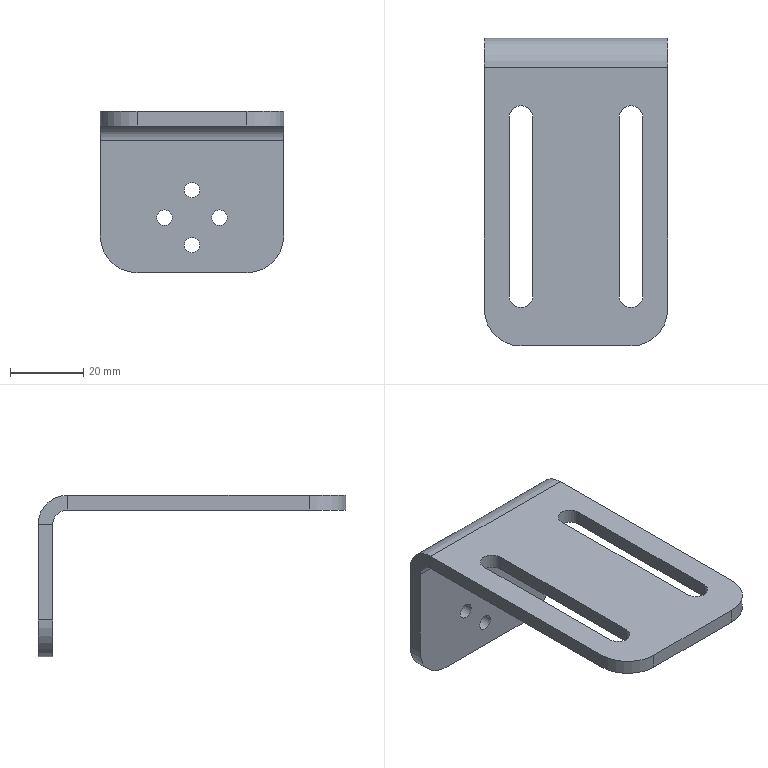Part | STEP file | JBJ-P-1010-04 | 1 solid | 30 faces | box 50 x 84 x 44 mm | volume 20932 mm3 | plane 16 | cylinder 14 | commonest cylinder face diameters 4.2 x4 6.5 x4 20 x4 8 x1 16 x1
STEP:
#1=CARTESIAN_POINT('',(50.,-4.,40.));
#2=VERTEX_POINT('',#1);
#3=CARTESIAN_POINT('',(50.,-4.,44.));
#4=VERTEX_POINT('',#3);
#5=CARTESIAN_POINT('',(50.,-4.,40.));
#6=DIRECTION('',(0.,0.,1.));
#7=VECTOR('',#6,1000.);
#8=LINE('',#5,#7);
#9=EDGE_CURVE('',#2,#4,#8,.T.);
#10=ORIENTED_EDGE('',*,*,#9,.F.);
#11=CARTESIAN_POINT('',(50.,0.,36.));
#12=VERTEX_POINT('',#11);
#13=CARTESIAN_POINT('',(50.,-4.,36.));
#14=DIRECTION('',(1.,0.,0.));
#15=DIRECTION('',(0.,0.,1.));
#16=AXIS2_PLACEMENT_3D('',#13,#14,#15);
#17=CIRCLE('',#16,4.);
#18=EDGE_CURVE('',#12,#2,#17,.T.);
#19=ORIENTED_EDGE('',*,*,#18,.F.);
#20=CARTESIAN_POINT('',(50.,4.,36.));
#21=VERTEX_POINT('',#20);
#22=CARTESIAN_POINT('',(50.,4.,36.));
#23=DIRECTION('',(0.,-1.,0.));
#24=VECTOR('',#23,1000.);
#25=LINE('',#22,#24);
#26=EDGE_CURVE('',#21,#12,#25,.T.);
#27=ORIENTED_EDGE('',*,*,#26,.F.);
#28=CARTESIAN_POINT('',(50.,-4.,36.));
#29=DIRECTION('',(1.,0.,0.));
#30=DIRECTION('',(0.,0.,-1.));
#31=AXIS2_PLACEMENT_3D('',#28,#29,#30);
#32=CIRCLE('',#31,8.);
#33=EDGE_CURVE('',#21,#4,#32,.T.);
#34=ORIENTED_EDGE('',*,*,#33,.T.);
#35=EDGE_LOOP('',(#10,#19,#27,#34));
#36=FACE_OUTER_BOUND('',#35,.T.);
#37=CARTESIAN_POINT('',(50.,-4.,40.));
#38=DIRECTION('',(1.,0.,0.));
#39=DIRECTION('',(0.,0.,-1.));
#40=AXIS2_PLACEMENT_3D('',#37,#38,#39);
#41=PLANE('',#40);
#42=ADVANCED_FACE('',(#36),#41,.T.);
#43=CARTESIAN_POINT('',(50.,-70.,44.));
#44=VERTEX_POINT('',#43);
#45=CARTESIAN_POINT('',(50.,0.,44.));
#46=DIRECTION('',(0.,-1.,0.));
#47=VECTOR('',#46,1000.);
#48=LINE('',#45,#47);
#49=EDGE_CURVE('',#4,#44,#48,.T.);
#50=ORIENTED_EDGE('',*,*,#49,.T.);
#51=CARTESIAN_POINT('',(50.,-70.,40.));
#52=VERTEX_POINT('',#51);
#53=CARTESIAN_POINT('',(50.,-70.,36.));
#54=DIRECTION('',(0.,0.,-1.));
#55=VECTOR('',#54,1000.);
#56=LINE('',#53,#55);
#57=EDGE_CURVE('',#44,#52,#56,.T.);
#58=ORIENTED_EDGE('',*,*,#57,.T.);
#59=CARTESIAN_POINT('',(50.,0.,40.));
#60=DIRECTION('',(0.,-1.,0.));
#61=VECTOR('',#60,1000.);
#62=LINE('',#59,#61);
#63=EDGE_CURVE('',#2,#52,#62,.T.);
#64=ORIENTED_EDGE('',*,*,#63,.F.);
#65=ORIENTED_EDGE('',*,*,#9,.T.);
#66=EDGE_LOOP('',(#50,#58,#64,#65));
#67=FACE_OUTER_BOUND('',#66,.T.);
#68=CARTESIAN_POINT('',(50.,4.,36.));
#69=DIRECTION('',(1.,0.,0.));
#70=DIRECTION('',(0.,0.,-1.));
#71=AXIS2_PLACEMENT_3D('',#68,#69,#70);
#72=PLANE('',#71);
#73=ADVANCED_FACE('',(#67),#72,.T.);
#74=CARTESIAN_POINT('',(0.,0.,36.));
#75=VERTEX_POINT('',#74);
#76=CARTESIAN_POINT('',(0.,4.,36.));
#77=VERTEX_POINT('',#76);
#78=CARTESIAN_POINT('',(0.,0.,36.));
#79=DIRECTION('',(0.,1.,0.));
#80=VECTOR('',#79,1000.);
#81=LINE('',#78,#80);
#82=EDGE_CURVE('',#75,#77,#81,.T.);
#83=ORIENTED_EDGE('',*,*,#82,.F.);
#84=CARTESIAN_POINT('',(0.,-4.,40.));
#85=VERTEX_POINT('',#84);
#86=CARTESIAN_POINT('',(0.,-4.,36.));
#87=DIRECTION('',(1.,0.,0.));
#88=DIRECTION('',(0.,0.,1.));
#89=AXIS2_PLACEMENT_3D('',#86,#87,#88);
#90=CIRCLE('',#89,4.);
#91=EDGE_CURVE('',#75,#85,#90,.T.);
#92=ORIENTED_EDGE('',*,*,#91,.T.);
#93=CARTESIAN_POINT('',(0.,-4.,44.));
#94=VERTEX_POINT('',#93);
#95=CARTESIAN_POINT('',(0.,-4.,44.));
#96=DIRECTION('',(0.,0.,-1.));
#97=VECTOR('',#96,1000.);
#98=LINE('',#95,#97);
#99=EDGE_CURVE('',#94,#85,#98,.T.);
#100=ORIENTED_EDGE('',*,*,#99,.F.);
#101=CARTESIAN_POINT('',(0.,-4.,36.));
#102=DIRECTION('',(1.,0.,0.));
#103=DIRECTION('',(0.,0.,-1.));
#104=AXIS2_PLACEMENT_3D('',#101,#102,#103);
#105=CIRCLE('',#104,8.);
#106=EDGE_CURVE('',#77,#94,#105,.T.);
#107=ORIENTED_EDGE('',*,*,#106,.F.);
#108=EDGE_LOOP('',(#83,#92,#100,#107));
#109=FACE_OUTER_BOUND('',#108,.T.);
#110=CARTESIAN_POINT('',(0.,0.,36.));
#111=DIRECTION('',(-1.,0.,0.));
#112=DIRECTION('',(0.,0.,1.));
#113=AXIS2_PLACEMENT_3D('',#110,#111,#112);
#114=PLANE('',#113);
#115=ADVANCED_FACE('',(#109),#114,.T.);
#116=CARTESIAN_POINT('',(0.,4.,10.));
#117=VERTEX_POINT('',#116);
#118=CARTESIAN_POINT('',(0.,4.,0.));
#119=DIRECTION('',(0.,0.,1.));
#120=VECTOR('',#119,1000.);
#121=LINE('',#118,#120);
#122=EDGE_CURVE('',#117,#77,#121,.T.);
#123=ORIENTED_EDGE('',*,*,#122,.F.);
#124=CARTESIAN_POINT('',(0.,0.,10.));
#125=VERTEX_POINT('',#124);
#126=CARTESIAN_POINT('',(0.,-4.,10.));
#127=DIRECTION('',(0.,-1.,0.));
#128=VECTOR('',#127,1000.);
#129=LINE('',#126,#128);
#130=EDGE_CURVE('',#117,#125,#129,.T.);
#131=ORIENTED_EDGE('',*,*,#130,.T.);
#132=CARTESIAN_POINT('',(0.,0.,0.));
#133=DIRECTION('',(0.,0.,1.));
#134=VECTOR('',#133,1000.);
#135=LINE('',#132,#134);
#136=EDGE_CURVE('',#125,#75,#135,.T.);
#137=ORIENTED_EDGE('',*,*,#136,.T.);
#138=ORIENTED_EDGE('',*,*,#82,.T.);
#139=EDGE_LOOP('',(#123,#131,#137,#138));
#140=FACE_OUTER_BOUND('',#139,.T.);
#141=CARTESIAN_POINT('',(0.,-4.,44.));
#142=DIRECTION('',(-1.,0.,0.));
#143=DIRECTION('',(0.,0.,1.));
#144=AXIS2_PLACEMENT_3D('',#141,#142,#143);
#145=PLANE('',#144);
#146=ADVANCED_FACE('',(#140),#145,.T.);
#147=CARTESIAN_POINT('',(36.75,-17.75,44.));
#148=VERTEX_POINT('',#147);
#149=CARTESIAN_POINT('',(43.25,-17.75,44.));
#150=VERTEX_POINT('',#149);
#151=CARTESIAN_POINT('',(40.,-17.75,44.));
#152=DIRECTION('',(0.,0.,-1.));
#153=DIRECTION('',(0.,1.,0.));
#154=AXIS2_PLACEMENT_3D('',#151,#152,#153);
#155=CIRCLE('',#154,3.25);
#156=EDGE_CURVE('',#148,#150,#155,.T.);
#157=ORIENTED_EDGE('',*,*,#156,.T.);
#158=CARTESIAN_POINT('',(43.25,-66.25,44.));
#159=VERTEX_POINT('',#158);
#160=CARTESIAN_POINT('',(43.25,-17.75,44.));
#161=DIRECTION('',(0.,-1.,0.));
#162=VECTOR('',#161,1000.);
#163=LINE('',#160,#162);
#164=EDGE_CURVE('',#150,#159,#163,.T.);
#165=ORIENTED_EDGE('',*,*,#164,.T.);
#166=CARTESIAN_POINT('',(36.75,-66.25,44.));
#167=VERTEX_POINT('',#166);
#168=CARTESIAN_POINT('',(40.,-66.25,44.));
#169=DIRECTION('',(0.,0.,-1.));
#170=DIRECTION('',(0.,1.,0.));
#171=AXIS2_PLACEMENT_3D('',#168,#169,#170);
#172=CIRCLE('',#171,3.25);
#173=EDGE_CURVE('',#159,#167,#172,.T.);
#174=ORIENTED_EDGE('',*,*,#173,.T.);
#175=CARTESIAN_POINT('',(36.75,-17.75,44.));
#176=DIRECTION('',(0.,-1.,0.));
#177=VECTOR('',#176,1000.);
#178=LINE('',#175,#177);
#179=EDGE_CURVE('',#148,#167,#178,.T.);
#180=ORIENTED_EDGE('',*,*,#179,.F.);
#181=EDGE_LOOP('',(#157,#165,#174,#180));
#182=FACE_BOUND('',#181,.T.);
#183=CARTESIAN_POINT('',(6.75,-17.75,44.));
#184=VERTEX_POINT('',#183);
#185=CARTESIAN_POINT('',(6.75,-66.25,44.));
#186=VERTEX_POINT('',#185);
#187=CARTESIAN_POINT('',(6.75,-17.75,44.));
#188=DIRECTION('',(0.,-1.,0.));
#189=VECTOR('',#188,1000.);
#190=LINE('',#187,#189);
#191=EDGE_CURVE('',#184,#186,#190,.T.);
#192=ORIENTED_EDGE('',*,*,#191,.F.);
#193=CARTESIAN_POINT('',(13.25,-17.75,44.));
#194=VERTEX_POINT('',#193);
#195=CARTESIAN_POINT('',(10.,-17.75,44.));
#196=DIRECTION('',(0.,0.,-1.));
#197=DIRECTION('',(0.,1.,0.));
#198=AXIS2_PLACEMENT_3D('',#195,#196,#197);
#199=CIRCLE('',#198,3.25);
#200=EDGE_CURVE('',#184,#194,#199,.T.);
#201=ORIENTED_EDGE('',*,*,#200,.T.);
#202=CARTESIAN_POINT('',(13.25,-66.25,44.));
#203=VERTEX_POINT('',#202);
#204=CARTESIAN_POINT('',(13.25,-17.75,44.));
#205=DIRECTION('',(0.,-1.,0.));
#206=VECTOR('',#205,1000.);
#207=LINE('',#204,#206);
#208=EDGE_CURVE('',#194,#203,#207,.T.);
#209=ORIENTED_EDGE('',*,*,#208,.T.);
#210=CARTESIAN_POINT('',(10.,-66.25,44.));
#211=DIRECTION('',(0.,0.,-1.));
#212=DIRECTION('',(0.,1.,0.));
#213=AXIS2_PLACEMENT_3D('',#210,#211,#212);
#214=CIRCLE('',#213,3.25);
#215=EDGE_CURVE('',#203,#186,#214,.T.);
#216=ORIENTED_EDGE('',*,*,#215,.T.);
#217=EDGE_LOOP('',(#192,#201,#209,#216));
#218=FACE_BOUND('',#217,.T.);
#219=CARTESIAN_POINT('',(40.,-80.,44.));
#220=VERTEX_POINT('',#219);
#221=CARTESIAN_POINT('',(10.,-80.,44.));
#222=VERTEX_POINT('',#221);
#223=CARTESIAN_POINT('',(50.,-80.,44.));
#224=DIRECTION('',(-1.,0.,0.));
#225=VECTOR('',#224,1000.);
#226=LINE('',#223,#225);
#227=EDGE_CURVE('',#220,#222,#226,.T.);
#228=ORIENTED_EDGE('',*,*,#227,.F.);
#229=CARTESIAN_POINT('',(40.,-70.,44.));
#230=DIRECTION('',(0.,0.,1.));
#231=DIRECTION('',(0.,1.,0.));
#232=AXIS2_PLACEMENT_3D('',#229,#230,#231);
#233=CIRCLE('',#232,10.);
#234=EDGE_CURVE('',#220,#44,#233,.T.);
#235=ORIENTED_EDGE('',*,*,#234,.T.);
#236=ORIENTED_EDGE('',*,*,#49,.F.);
#237=CARTESIAN_POINT('',(50.,-4.,44.));
#238=DIRECTION('',(-1.,0.,0.));
#239=VECTOR('',#238,1000.);
#240=LINE('',#237,#239);
#241=EDGE_CURVE('',#4,#94,#240,.T.);
#242=ORIENTED_EDGE('',*,*,#241,.T.);
#243=CARTESIAN_POINT('',(0.,-70.,44.));
#244=VERTEX_POINT('',#243);
#245=CARTESIAN_POINT('',(0.,0.,44.));
#246=DIRECTION('',(0.,-1.,0.));
#247=VECTOR('',#246,1000.);
#248=LINE('',#245,#247);
#249=EDGE_CURVE('',#94,#244,#248,.T.);
#250=ORIENTED_EDGE('',*,*,#249,.T.);
#251=CARTESIAN_POINT('',(10.,-70.,44.));
#252=DIRECTION('',(0.,0.,1.));
#253=DIRECTION('',(0.,1.,0.));
#254=AXIS2_PLACEMENT_3D('',#251,#252,#253);
#255=CIRCLE('',#254,10.);
#256=EDGE_CURVE('',#244,#222,#255,.T.);
#257=ORIENTED_EDGE('',*,*,#256,.T.);
#258=EDGE_LOOP('',(#228,#235,#236,#242,#250,#257));
#259=FACE_OUTER_BOUND('',#258,.T.);
#260=CARTESIAN_POINT('',(50.,0.,44.));
#261=DIRECTION('',(0.,0.,-1.));
#262=DIRECTION('',(0.,1.,0.));
#263=AXIS2_PLACEMENT_3D('',#260,#261,#262);
#264=PLANE('',#263);
#265=ADVANCED_FACE('',(#182,#218,#259),#264,.F.);
#266=CARTESIAN_POINT('',(40.,-80.,40.));
#267=VERTEX_POINT('',#266);
#268=CARTESIAN_POINT('',(10.,-80.,40.));
#269=VERTEX_POINT('',#268);
#270=CARTESIAN_POINT('',(50.,-80.,40.));
#271=DIRECTION('',(-1.,0.,0.));
#272=VECTOR('',#271,1000.);
#273=LINE('',#270,#272);
#274=EDGE_CURVE('',#267,#269,#273,.T.);
#275=ORIENTED_EDGE('',*,*,#274,.F.);
#276=CARTESIAN_POINT('',(40.,-80.,40.));
#277=DIRECTION('',(0.,0.,1.));
#278=VECTOR('',#277,1000.);
#279=LINE('',#276,#278);
#280=EDGE_CURVE('',#267,#220,#279,.T.);
#281=ORIENTED_EDGE('',*,*,#280,.T.);
#282=ORIENTED_EDGE('',*,*,#227,.T.);
#283=CARTESIAN_POINT('',(10.,-80.,40.));
#284=DIRECTION('',(0.,0.,-1.));
#285=VECTOR('',#284,1000.);
#286=LINE('',#283,#285);
#287=EDGE_CURVE('',#222,#269,#286,.T.);
#288=ORIENTED_EDGE('',*,*,#287,.T.);
#289=EDGE_LOOP('',(#275,#281,#282,#288));
#290=FACE_OUTER_BOUND('',#289,.T.);
#291=CARTESIAN_POINT('',(50.,-80.,40.));
#292=DIRECTION('',(0.,-1.,0.));
#293=DIRECTION('',(0.,0.,-1.));
#294=AXIS2_PLACEMENT_3D('',#291,#292,#293);
#295=PLANE('',#294);
#296=ADVANCED_FACE('',(#290),#295,.T.);
#297=CARTESIAN_POINT('',(36.75,-17.75,40.));
#298=VERTEX_POINT('',#297);
#299=CARTESIAN_POINT('',(36.75,-66.25,40.));
#300=VERTEX_POINT('',#299);
#301=CARTESIAN_POINT('',(36.75,-17.75,40.));
#302=DIRECTION('',(0.,-1.,0.));
#303=VECTOR('',#302,1000.);
#304=LINE('',#301,#303);
#305=EDGE_CURVE('',#298,#300,#304,.T.);
#306=ORIENTED_EDGE('',*,*,#305,.T.);
#307=CARTESIAN_POINT('',(43.25,-66.25,40.));
#308=VERTEX_POINT('',#307);
#309=CARTESIAN_POINT('',(40.,-66.25,40.));
#310=DIRECTION('',(0.,0.,-1.));
#311=DIRECTION('',(0.,1.,0.));
#312=AXIS2_PLACEMENT_3D('',#309,#310,#311);
#313=CIRCLE('',#312,3.25);
#314=EDGE_CURVE('',#308,#300,#313,.T.);
#315=ORIENTED_EDGE('',*,*,#314,.F.);
#316=CARTESIAN_POINT('',(43.25,-17.75,40.));
#317=VERTEX_POINT('',#316);
#318=CARTESIAN_POINT('',(43.25,-17.75,40.));
#319=DIRECTION('',(0.,-1.,0.));
#320=VECTOR('',#319,1000.);
#321=LINE('',#318,#320);
#322=EDGE_CURVE('',#317,#308,#321,.T.);
#323=ORIENTED_EDGE('',*,*,#322,.F.);
#324=CARTESIAN_POINT('',(40.,-17.75,40.));
#325=DIRECTION('',(0.,0.,-1.));
#326=DIRECTION('',(0.,1.,0.));
#327=AXIS2_PLACEMENT_3D('',#324,#325,#326);
#328=CIRCLE('',#327,3.25);
#329=EDGE_CURVE('',#298,#317,#328,.T.);
#330=ORIENTED_EDGE('',*,*,#329,.F.);
#331=EDGE_LOOP('',(#306,#315,#323,#330));
#332=FACE_BOUND('',#331,.T.);
#333=CARTESIAN_POINT('',(13.25,-17.75,40.));
#334=VERTEX_POINT('',#333);
#335=CARTESIAN_POINT('',(13.25,-66.25,40.));
#336=VERTEX_POINT('',#335);
#337=CARTESIAN_POINT('',(13.25,-17.75,40.));
#338=DIRECTION('',(0.,-1.,0.));
#339=VECTOR('',#338,1000.);
#340=LINE('',#337,#339);
#341=EDGE_CURVE('',#334,#336,#340,.T.);
#342=ORIENTED_EDGE('',*,*,#341,.F.);
#343=CARTESIAN_POINT('',(6.75,-17.75,40.));
#344=VERTEX_POINT('',#343);
#345=CARTESIAN_POINT('',(10.,-17.75,40.));
#346=DIRECTION('',(0.,0.,-1.));
#347=DIRECTION('',(0.,1.,0.));
#348=AXIS2_PLACEMENT_3D('',#345,#346,#347);
#349=CIRCLE('',#348,3.25);
#350=EDGE_CURVE('',#344,#334,#349,.T.);
#351=ORIENTED_EDGE('',*,*,#350,.F.);
#352=CARTESIAN_POINT('',(6.75,-66.25,40.));
#353=VERTEX_POINT('',#352);
#354=CARTESIAN_POINT('',(6.75,-17.75,40.));
#355=DIRECTION('',(0.,-1.,0.));
#356=VECTOR('',#355,1000.);
#357=LINE('',#354,#356);
#358=EDGE_CURVE('',#344,#353,#357,.T.);
#359=ORIENTED_EDGE('',*,*,#358,.T.);
#360=CARTESIAN_POINT('',(10.,-66.25,40.));
#361=DIRECTION('',(0.,0.,-1.));
#362=DIRECTION('',(0.,1.,0.));
#363=AXIS2_PLACEMENT_3D('',#360,#361,#362);
#364=CIRCLE('',#363,3.25);
#365=EDGE_CURVE('',#336,#353,#364,.T.);
#366=ORIENTED_EDGE('',*,*,#365,.F.);
#367=EDGE_LOOP('',(#342,#351,#359,#366));
#368=FACE_BOUND('',#367,.T.);
#369=ORIENTED_EDGE('',*,*,#63,.T.);
#370=CARTESIAN_POINT('',(40.,-70.,40.));
#371=DIRECTION('',(0.,0.,-1.));
#372=DIRECTION('',(0.,1.,0.));
#373=AXIS2_PLACEMENT_3D('',#370,#371,#372);
#374=CIRCLE('',#373,10.);
#375=EDGE_CURVE('',#52,#267,#374,.T.);
#376=ORIENTED_EDGE('',*,*,#375,.T.);
#377=ORIENTED_EDGE('',*,*,#274,.T.);
#378=CARTESIAN_POINT('',(0.,-70.,40.));
#379=VERTEX_POINT('',#378);
#380=CARTESIAN_POINT('',(10.,-70.,40.));
#381=DIRECTION('',(0.,0.,-1.));
#382=DIRECTION('',(0.,1.,0.));
#383=AXIS2_PLACEMENT_3D('',#380,#381,#382);
#384=CIRCLE('',#383,10.);
#385=EDGE_CURVE('',#269,#379,#384,.T.);
#386=ORIENTED_EDGE('',*,*,#385,.T.);
#387=CARTESIAN_POINT('',(0.,0.,40.));
#388=DIRECTION('',(0.,-1.,0.));
#389=VECTOR('',#388,1000.);
#390=LINE('',#387,#389);
#391=EDGE_CURVE('',#85,#379,#390,.T.);
#392=ORIENTED_EDGE('',*,*,#391,.F.);
#393=CARTESIAN_POINT('',(50.,-4.,40.));
#394=DIRECTION('',(-1.,0.,0.));
#395=VECTOR('',#394,1000.);
#396=LINE('',#393,#395);
#397=EDGE_CURVE('',#2,#85,#396,.T.);
#398=ORIENTED_EDGE('',*,*,#397,.F.);
#399=EDGE_LOOP('',(#369,#376,#377,#386,#392,#398));
#400=FACE_OUTER_BOUND('',#399,.T.);
#401=CARTESIAN_POINT('',(50.,0.,40.));
#402=DIRECTION('',(0.,0.,-1.));
#403=DIRECTION('',(0.,1.,0.));
#404=AXIS2_PLACEMENT_3D('',#401,#402,#403);
#405=PLANE('',#404);
#406=ADVANCED_FACE('',(#332,#368,#400),#405,.T.);
#407=ORIENTED_EDGE('',*,*,#91,.F.);
#408=CARTESIAN_POINT('',(50.,0.,36.));
#409=DIRECTION('',(-1.,0.,0.));
#410=VECTOR('',#409,1000.);
#411=LINE('',#408,#410);
#412=EDGE_CURVE('',#12,#75,#411,.T.);
#413=ORIENTED_EDGE('',*,*,#412,.F.);
#414=ORIENTED_EDGE('',*,*,#18,.T.);
#415=ORIENTED_EDGE('',*,*,#397,.T.);
#416=EDGE_LOOP('',(#407,#413,#414,#415));
#417=FACE_OUTER_BOUND('',#416,.T.);
#418=CARTESIAN_POINT('',(50.,-4.,36.));
#419=DIRECTION('',(-1.,0.,0.));
#420=DIRECTION('',(0.,0.,1.));
#421=AXIS2_PLACEMENT_3D('',#418,#419,#420);
#422=CYLINDRICAL_SURFACE('',#421,4.);
#423=ADVANCED_FACE('',(#417),#422,.F.);
#424=CARTESIAN_POINT('',(25.,0.,20.4));
#425=VERTEX_POINT('',#424);
#426=CARTESIAN_POINT('',(25.,0.,22.5));
#427=DIRECTION('',(0.,-1.,0.));
#428=DIRECTION('',(0.,0.,-1.));
#429=AXIS2_PLACEMENT_3D('',#426,#427,#428);
#430=CIRCLE('',#429,2.1);
#431=EDGE_CURVE('',#425,#425,#430,.T.);
#432=ORIENTED_EDGE('',*,*,#431,.F.);
#433=EDGE_LOOP('',(#432));
#434=FACE_BOUND('',#433,.T.);
#435=CARTESIAN_POINT('',(17.5,0.,12.9));
#436=VERTEX_POINT('',#435);
#437=CARTESIAN_POINT('',(17.5,0.,15.));
#438=DIRECTION('',(0.,-1.,0.));
#439=DIRECTION('',(0.,0.,-1.));
#440=AXIS2_PLACEMENT_3D('',#437,#438,#439);
#441=CIRCLE('',#440,2.1);
#442=EDGE_CURVE('',#436,#436,#441,.T.);
#443=ORIENTED_EDGE('',*,*,#442,.F.);
#444=EDGE_LOOP('',(#443));
#445=FACE_BOUND('',#444,.T.);
#446=CARTESIAN_POINT('',(25.,0.,5.4));
#447=VERTEX_POINT('',#446);
#448=CARTESIAN_POINT('',(25.,0.,7.5));
#449=DIRECTION('',(0.,-1.,0.));
#450=DIRECTION('',(0.,0.,-1.));
#451=AXIS2_PLACEMENT_3D('',#448,#449,#450);
#452=CIRCLE('',#451,2.1);
#453=EDGE_CURVE('',#447,#447,#452,.T.);
#454=ORIENTED_EDGE('',*,*,#453,.F.);
#455=EDGE_LOOP('',(#454));
#456=FACE_BOUND('',#455,.T.);
#457=CARTESIAN_POINT('',(32.5,0.,12.9));
#458=VERTEX_POINT('',#457);
#459=CARTESIAN_POINT('',(32.5,0.,15.));
#460=DIRECTION('',(0.,-1.,0.));
#461=DIRECTION('',(0.,0.,-1.));
#462=AXIS2_PLACEMENT_3D('',#459,#460,#461);
#463=CIRCLE('',#462,2.1);
#464=EDGE_CURVE('',#458,#458,#463,.T.);
#465=ORIENTED_EDGE('',*,*,#464,.F.);
#466=EDGE_LOOP('',(#465));
#467=FACE_BOUND('',#466,.T.);
#468=ORIENTED_EDGE('',*,*,#136,.F.);
#469=CARTESIAN_POINT('',(10.,0.,0.));
#470=VERTEX_POINT('',#469);
#471=CARTESIAN_POINT('',(10.,0.,10.));
#472=DIRECTION('',(0.,-1.,0.));
#473=DIRECTION('',(0.,0.,-1.));
#474=AXIS2_PLACEMENT_3D('',#471,#472,#473);
#475=CIRCLE('',#474,10.);
#476=EDGE_CURVE('',#125,#470,#475,.T.);
#477=ORIENTED_EDGE('',*,*,#476,.T.);
#478=CARTESIAN_POINT('',(40.,0.,0.));
#479=VERTEX_POINT('',#478);
#480=CARTESIAN_POINT('',(50.,0.,0.));
#481=DIRECTION('',(-1.,0.,0.));
#482=VECTOR('',#481,1000.);
#483=LINE('',#480,#482);
#484=EDGE_CURVE('',#479,#470,#483,.T.);
#485=ORIENTED_EDGE('',*,*,#484,.F.);
#486=CARTESIAN_POINT('',(50.,0.,10.));
#487=VERTEX_POINT('',#486);
#488=CARTESIAN_POINT('',(40.,0.,10.));
#489=DIRECTION('',(0.,-1.,0.));
#490=DIRECTION('',(0.,0.,-1.));
#491=AXIS2_PLACEMENT_3D('',#488,#489,#490);
#492=CIRCLE('',#491,10.);
#493=EDGE_CURVE('',#479,#487,#492,.T.);
#494=ORIENTED_EDGE('',*,*,#493,.T.);
#495=CARTESIAN_POINT('',(50.,0.,0.));
#496=DIRECTION('',(0.,0.,1.));
#497=VECTOR('',#496,1000.);
#498=LINE('',#495,#497);
#499=EDGE_CURVE('',#487,#12,#498,.T.);
#500=ORIENTED_EDGE('',*,*,#499,.T.);
#501=ORIENTED_EDGE('',*,*,#412,.T.);
#502=EDGE_LOOP('',(#468,#477,#485,#494,#500,#501));
#503=FACE_OUTER_BOUND('',#502,.T.);
#504=CARTESIAN_POINT('',(50.,0.,0.));
#505=DIRECTION('',(0.,-1.,0.));
#506=DIRECTION('',(0.,0.,-1.));
#507=AXIS2_PLACEMENT_3D('',#504,#505,#506);
#508=PLANE('',#507);
#509=ADVANCED_FACE('',(#434,#445,#456,#467,#503),#508,.T.);
#510=ORIENTED_EDGE('',*,*,#484,.T.);
#511=CARTESIAN_POINT('',(10.,4.,0.));
#512=VERTEX_POINT('',#511);
#513=CARTESIAN_POINT('',(10.,4.,0.));
#514=DIRECTION('',(0.,1.,0.));
#515=VECTOR('',#514,1000.);
#516=LINE('',#513,#515);
#517=EDGE_CURVE('',#470,#512,#516,.T.);
#518=ORIENTED_EDGE('',*,*,#517,.T.);
#519=CARTESIAN_POINT('',(40.,4.,0.));
#520=VERTEX_POINT('',#519);
#521=CARTESIAN_POINT('',(50.,4.,0.));
#522=DIRECTION('',(-1.,0.,0.));
#523=VECTOR('',#522,1000.);
#524=LINE('',#521,#523);
#525=EDGE_CURVE('',#520,#512,#524,.T.);
#526=ORIENTED_EDGE('',*,*,#525,.F.);
#527=CARTESIAN_POINT('',(40.,0.,0.));
#528=DIRECTION('',(0.,-1.,0.));
#529=VECTOR('',#528,1000.);
#530=LINE('',#527,#529);
#531=EDGE_CURVE('',#520,#479,#530,.T.);
#532=ORIENTED_EDGE('',*,*,#531,.T.);
#533=EDGE_LOOP('',(#510,#518,#526,#532));
#534=FACE_OUTER_BOUND('',#533,.T.);
#535=CARTESIAN_POINT('',(50.,4.,0.));
#536=DIRECTION('',(0.,0.,-1.));
#537=DIRECTION('',(0.,1.,0.));
#538=AXIS2_PLACEMENT_3D('',#535,#536,#537);
#539=PLANE('',#538);
#540=ADVANCED_FACE('',(#534),#539,.T.);
#541=CARTESIAN_POINT('',(25.,4.,20.4));
#542=VERTEX_POINT('',#541);
#543=CARTESIAN_POINT('',(25.,4.,22.5));
#544=DIRECTION('',(0.,-1.,0.));
#545=DIRECTION('',(0.,0.,-1.));
#546=AXIS2_PLACEMENT_3D('',#543,#544,#545);
#547=CIRCLE('',#546,2.1);
#548=EDGE_CURVE('',#542,#542,#547,.T.);
#549=ORIENTED_EDGE('',*,*,#548,.T.);
#550=EDGE_LOOP('',(#549));
#551=FACE_BOUND('',#550,.T.);
#552=CARTESIAN_POINT('',(17.5,4.,12.9));
#553=VERTEX_POINT('',#552);
#554=CARTESIAN_POINT('',(17.5,4.,15.));
#555=DIRECTION('',(0.,-1.,0.));
#556=DIRECTION('',(0.,0.,-1.));
#557=AXIS2_PLACEMENT_3D('',#554,#555,#556);
#558=CIRCLE('',#557,2.1);
#559=EDGE_CURVE('',#553,#553,#558,.T.);
#560=ORIENTED_EDGE('',*,*,#559,.T.);
#561=EDGE_LOOP('',(#560));
#562=FACE_BOUND('',#561,.T.);
#563=CARTESIAN_POINT('',(25.,4.,5.4));
#564=VERTEX_POINT('',#563);
#565=CARTESIAN_POINT('',(25.,4.,7.5));
#566=DIRECTION('',(0.,-1.,0.));
#567=DIRECTION('',(0.,0.,-1.));
#568=AXIS2_PLACEMENT_3D('',#565,#566,#567);
#569=CIRCLE('',#568,2.1);
#570=EDGE_CURVE('',#564,#564,#569,.T.);
#571=ORIENTED_EDGE('',*,*,#570,.T.);
#572=EDGE_LOOP('',(#571));
#573=FACE_BOUND('',#572,.T.);
#574=CARTESIAN_POINT('',(32.5,4.,12.9));
#575=VERTEX_POINT('',#574);
#576=CARTESIAN_POINT('',(32.5,4.,15.));
#577=DIRECTION('',(0.,-1.,0.));
#578=DIRECTION('',(0.,0.,-1.));
#579=AXIS2_PLACEMENT_3D('',#576,#577,#578);
#580=CIRCLE('',#579,2.1);
#581=EDGE_CURVE('',#575,#575,#580,.T.);
#582=ORIENTED_EDGE('',*,*,#581,.T.);
#583=EDGE_LOOP('',(#582));
#584=FACE_BOUND('',#583,.T.);
#585=ORIENTED_EDGE('',*,*,#525,.T.);
#586=CARTESIAN_POINT('',(10.,4.,10.));
#587=DIRECTION('',(0.,1.,0.));
#588=DIRECTION('',(0.,0.,-1.));
#589=AXIS2_PLACEMENT_3D('',#586,#587,#588);
#590=CIRCLE('',#589,10.);
#591=EDGE_CURVE('',#512,#117,#590,.T.);
#592=ORIENTED_EDGE('',*,*,#591,.T.);
#593=ORIENTED_EDGE('',*,*,#122,.T.);
#594=CARTESIAN_POINT('',(50.,4.,36.));
#595=DIRECTION('',(-1.,0.,0.));
#596=VECTOR('',#595,1000.);
#597=LINE('',#594,#596);
#598=EDGE_CURVE('',#21,#77,#597,.T.);
#599=ORIENTED_EDGE('',*,*,#598,.F.);
#600=CARTESIAN_POINT('',(50.,4.,10.));
#601=VERTEX_POINT('',#600);
#602=CARTESIAN_POINT('',(50.,4.,0.));
#603=DIRECTION('',(0.,0.,1.));
#604=VECTOR('',#603,1000.);
#605=LINE('',#602,#604);
#606=EDGE_CURVE('',#601,#21,#605,.T.);
#607=ORIENTED_EDGE('',*,*,#606,.F.);
#608=CARTESIAN_POINT('',(40.,4.,10.));
#609=DIRECTION('',(0.,1.,0.));
#610=DIRECTION('',(0.,0.,-1.));
#611=AXIS2_PLACEMENT_3D('',#608,#609,#610);
#612=CIRCLE('',#611,10.);
#613=EDGE_CURVE('',#601,#520,#612,.T.);
#614=ORIENTED_EDGE('',*,*,#613,.T.);
#615=EDGE_LOOP('',(#585,#592,#593,#599,#607,#614));
#616=FACE_OUTER_BOUND('',#615,.T.);
#617=CARTESIAN_POINT('',(50.,4.,0.));
#618=DIRECTION('',(0.,-1.,0.));
#619=DIRECTION('',(0.,0.,-1.));
#620=AXIS2_PLACEMENT_3D('',#617,#618,#619);
#621=PLANE('',#620);
#622=ADVANCED_FACE('',(#551,#562,#573,#584,#616),#621,.F.);
#623=ORIENTED_EDGE('',*,*,#106,.T.);
#624=ORIENTED_EDGE('',*,*,#241,.F.);
#625=ORIENTED_EDGE('',*,*,#33,.F.);
#626=ORIENTED_EDGE('',*,*,#598,.T.);
#627=EDGE_LOOP('',(#623,#624,#625,#626));
#628=FACE_OUTER_BOUND('',#627,.T.);
#629=CARTESIAN_POINT('',(50.,-4.,36.));
#630=DIRECTION('',(-1.,0.,0.));
#631=DIRECTION('',(0.,0.,1.));
#632=AXIS2_PLACEMENT_3D('',#629,#630,#631);
#633=CYLINDRICAL_SURFACE('',#632,8.);
#634=ADVANCED_FACE('',(#628),#633,.T.);
#635=ORIENTED_EDGE('',*,*,#499,.F.);
#636=CARTESIAN_POINT('',(50.,4.,10.));
#637=DIRECTION('',(0.,1.,0.));
#638=VECTOR('',#637,1000.);
#639=LINE('',#636,#638);
#640=EDGE_CURVE('',#487,#601,#639,.T.);
#641=ORIENTED_EDGE('',*,*,#640,.T.);
#642=ORIENTED_EDGE('',*,*,#606,.T.);
#643=ORIENTED_EDGE('',*,*,#26,.T.);
#644=EDGE_LOOP('',(#635,#641,#642,#643));
#645=FACE_OUTER_BOUND('',#644,.T.);
#646=CARTESIAN_POINT('',(50.,-4.,36.));
#647=DIRECTION('',(-1.,0.,0.));
#648=DIRECTION('',(0.,0.,1.));
#649=AXIS2_PLACEMENT_3D('',#646,#647,#648);
#650=PLANE('',#649);
#651=ADVANCED_FACE('',(#645),#650,.F.);
#652=ORIENTED_EDGE('',*,*,#391,.T.);
#653=CARTESIAN_POINT('',(0.,-70.,36.));
#654=DIRECTION('',(0.,0.,1.));
#655=VECTOR('',#654,1000.);
#656=LINE('',#653,#655);
#657=EDGE_CURVE('',#379,#244,#656,.T.);
#658=ORIENTED_EDGE('',*,*,#657,.T.);
#659=ORIENTED_EDGE('',*,*,#249,.F.);
#660=ORIENTED_EDGE('',*,*,#99,.T.);
#661=EDGE_LOOP('',(#652,#658,#659,#660));
#662=FACE_OUTER_BOUND('',#661,.T.);
#663=CARTESIAN_POINT('',(0.,-4.,36.));
#664=DIRECTION('',(-1.,0.,0.));
#665=DIRECTION('',(0.,0.,1.));
#666=AXIS2_PLACEMENT_3D('',#663,#664,#665);
#667=PLANE('',#666);
#668=ADVANCED_FACE('',(#662),#667,.T.);
#669=ORIENTED_EDGE('',*,*,#215,.F.);
#670=CARTESIAN_POINT('',(13.25,-66.25,44.));
#671=DIRECTION('',(0.,0.,1.));
#672=VECTOR('',#671,1000.);
#673=LINE('',#670,#672);
#674=EDGE_CURVE('',#336,#203,#673,.T.);
#675=ORIENTED_EDGE('',*,*,#674,.F.);
#676=ORIENTED_EDGE('',*,*,#365,.T.);
#677=CARTESIAN_POINT('',(6.75,-66.25,40.));
#678=DIRECTION('',(0.,0.,-1.));
#679=VECTOR('',#678,1000.);
#680=LINE('',#677,#679);
#681=EDGE_CURVE('',#186,#353,#680,.T.);
#682=ORIENTED_EDGE('',*,*,#681,.F.);
#683=EDGE_LOOP('',(#669,#675,#676,#682));
#684=FACE_OUTER_BOUND('',#683,.T.);
#685=CARTESIAN_POINT('',(10.,-66.25,40.));
#686=DIRECTION('',(0.,0.,-1.));
#687=DIRECTION('',(0.,1.,0.));
#688=AXIS2_PLACEMENT_3D('',#685,#686,#687);
#689=CYLINDRICAL_SURFACE('',#688,3.25);
#690=ADVANCED_FACE('',(#684),#689,.F.);
#691=ORIENTED_EDGE('',*,*,#350,.T.);
#692=CARTESIAN_POINT('',(13.25,-17.75,44.));
#693=DIRECTION('',(0.,0.,1.));
#694=VECTOR('',#693,1000.);
#695=LINE('',#692,#694);
#696=EDGE_CURVE('',#334,#194,#695,.T.);
#697=ORIENTED_EDGE('',*,*,#696,.T.);
#698=ORIENTED_EDGE('',*,*,#200,.F.);
#699=CARTESIAN_POINT('',(6.75,-17.75,40.));
#700=DIRECTION('',(0.,0.,1.));
#701=VECTOR('',#700,1000.);
#702=LINE('',#699,#701);
#703=EDGE_CURVE('',#344,#184,#702,.T.);
#704=ORIENTED_EDGE('',*,*,#703,.F.);
#705=EDGE_LOOP('',(#691,#697,#698,#704));
#706=FACE_OUTER_BOUND('',#705,.T.);
#707=CARTESIAN_POINT('',(10.,-17.75,40.));
#708=DIRECTION('',(0.,0.,-1.));
#709=DIRECTION('',(0.,1.,0.));
#710=AXIS2_PLACEMENT_3D('',#707,#708,#709);
#711=CYLINDRICAL_SURFACE('',#710,3.25);
#712=ADVANCED_FACE('',(#706),#711,.F.);
#713=ORIENTED_EDGE('',*,*,#681,.T.);
#714=ORIENTED_EDGE('',*,*,#358,.F.);
#715=ORIENTED_EDGE('',*,*,#703,.T.);
#716=ORIENTED_EDGE('',*,*,#191,.T.);
#717=EDGE_LOOP('',(#713,#714,#715,#716));
#718=FACE_OUTER_BOUND('',#717,.T.);
#719=CARTESIAN_POINT('',(6.75,-17.75,40.));
#720=DIRECTION('',(-1.,0.,0.));
#721=DIRECTION('',(0.,-1.,0.));
#722=AXIS2_PLACEMENT_3D('',#719,#720,#721);
#723=PLANE('',#722);
#724=ADVANCED_FACE('',(#718),#723,.F.);
#725=ORIENTED_EDGE('',*,*,#674,.T.);
#726=ORIENTED_EDGE('',*,*,#208,.F.);
#727=ORIENTED_EDGE('',*,*,#696,.F.);
#728=ORIENTED_EDGE('',*,*,#341,.T.);
#729=EDGE_LOOP('',(#725,#726,#727,#728));
#730=FACE_OUTER_BOUND('',#729,.T.);
#731=CARTESIAN_POINT('',(13.25,-17.75,44.));
#732=DIRECTION('',(1.,0.,0.));
#733=DIRECTION('',(0.,1.,0.));
#734=AXIS2_PLACEMENT_3D('',#731,#732,#733);
#735=PLANE('',#734);
#736=ADVANCED_FACE('',(#730),#735,.F.);
#737=ORIENTED_EDGE('',*,*,#173,.F.);
#738=CARTESIAN_POINT('',(43.25,-66.25,44.));
#739=DIRECTION('',(0.,0.,1.));
#740=VECTOR('',#739,1000.);
#741=LINE('',#738,#740);
#742=EDGE_CURVE('',#308,#159,#741,.T.);
#743=ORIENTED_EDGE('',*,*,#742,.F.);
#744=ORIENTED_EDGE('',*,*,#314,.T.);
#745=CARTESIAN_POINT('',(36.75,-66.25,40.));
#746=DIRECTION('',(0.,0.,-1.));
#747=VECTOR('',#746,1000.);
#748=LINE('',#745,#747);
#749=EDGE_CURVE('',#167,#300,#748,.T.);
#750=ORIENTED_EDGE('',*,*,#749,.F.);
#751=EDGE_LOOP('',(#737,#743,#744,#750));
#752=FACE_OUTER_BOUND('',#751,.T.);
#753=CARTESIAN_POINT('',(40.,-66.25,40.));
#754=DIRECTION('',(0.,0.,-1.));
#755=DIRECTION('',(0.,1.,0.));
#756=AXIS2_PLACEMENT_3D('',#753,#754,#755);
#757=CYLINDRICAL_SURFACE('',#756,3.25);
#758=ADVANCED_FACE('',(#752),#757,.F.);
#759=ORIENTED_EDGE('',*,*,#329,.T.);
#760=CARTESIAN_POINT('',(43.25,-17.75,44.));
#761=DIRECTION('',(0.,0.,1.));
#762=VECTOR('',#761,1000.);
#763=LINE('',#760,#762);
#764=EDGE_CURVE('',#317,#150,#763,.T.);
#765=ORIENTED_EDGE('',*,*,#764,.T.);
#766=ORIENTED_EDGE('',*,*,#156,.F.);
#767=CARTESIAN_POINT('',(36.75,-17.75,40.));
#768=DIRECTION('',(0.,0.,1.));
#769=VECTOR('',#768,1000.);
#770=LINE('',#767,#769);
#771=EDGE_CURVE('',#298,#148,#770,.T.);
#772=ORIENTED_EDGE('',*,*,#771,.F.);
#773=EDGE_LOOP('',(#759,#765,#766,#772));
#774=FACE_OUTER_BOUND('',#773,.T.);
#775=CARTESIAN_POINT('',(40.,-17.75,40.));
#776=DIRECTION('',(0.,0.,-1.));
#777=DIRECTION('',(0.,1.,0.));
#778=AXIS2_PLACEMENT_3D('',#775,#776,#777);
#779=CYLINDRICAL_SURFACE('',#778,3.25);
#780=ADVANCED_FACE('',(#774),#779,.F.);
#781=ORIENTED_EDGE('',*,*,#749,.T.);
#782=ORIENTED_EDGE('',*,*,#305,.F.);
#783=ORIENTED_EDGE('',*,*,#771,.T.);
#784=ORIENTED_EDGE('',*,*,#179,.T.);
#785=EDGE_LOOP('',(#781,#782,#783,#784));
#786=FACE_OUTER_BOUND('',#785,.T.);
#787=CARTESIAN_POINT('',(36.75,-17.75,40.));
#788=DIRECTION('',(-1.,0.,0.));
#789=DIRECTION('',(0.,0.,1.));
#790=AXIS2_PLACEMENT_3D('',#787,#788,#789);
#791=PLANE('',#790);
#792=ADVANCED_FACE('',(#786),#791,.F.);
#793=ORIENTED_EDGE('',*,*,#742,.T.);
#794=ORIENTED_EDGE('',*,*,#164,.F.);
#795=ORIENTED_EDGE('',*,*,#764,.F.);
#796=ORIENTED_EDGE('',*,*,#322,.T.);
#797=EDGE_LOOP('',(#793,#794,#795,#796));
#798=FACE_OUTER_BOUND('',#797,.T.);
#799=CARTESIAN_POINT('',(43.25,-17.75,44.));
#800=DIRECTION('',(1.,0.,0.));
#801=DIRECTION('',(0.,0.,-1.));
#802=AXIS2_PLACEMENT_3D('',#799,#800,#801);
#803=PLANE('',#802);
#804=ADVANCED_FACE('',(#798),#803,.F.);
#805=ORIENTED_EDGE('',*,*,#581,.F.);
#806=EDGE_LOOP('',(#805));
#807=FACE_OUTER_BOUND('',#806,.T.);
#808=ORIENTED_EDGE('',*,*,#464,.T.);
#809=EDGE_LOOP('',(#808));
#810=FACE_OUTER_BOUND('',#809,.T.);
#811=CARTESIAN_POINT('',(32.5,0.,15.));
#812=DIRECTION('',(0.,-1.,0.));
#813=DIRECTION('',(0.,0.,-1.));
#814=AXIS2_PLACEMENT_3D('',#811,#812,#813);
#815=CYLINDRICAL_SURFACE('',#814,2.1);
#816=ADVANCED_FACE('',(#807,#810),#815,.F.);
#817=ORIENTED_EDGE('',*,*,#570,.F.);
#818=EDGE_LOOP('',(#817));
#819=FACE_OUTER_BOUND('',#818,.T.);
#820=ORIENTED_EDGE('',*,*,#453,.T.);
#821=EDGE_LOOP('',(#820));
#822=FACE_OUTER_BOUND('',#821,.T.);
#823=CARTESIAN_POINT('',(25.,0.,7.5));
#824=DIRECTION('',(0.,-1.,0.));
#825=DIRECTION('',(0.,0.,-1.));
#826=AXIS2_PLACEMENT_3D('',#823,#824,#825);
#827=CYLINDRICAL_SURFACE('',#826,2.1);
#828=ADVANCED_FACE('',(#819,#822),#827,.F.);
#829=ORIENTED_EDGE('',*,*,#559,.F.);
#830=EDGE_LOOP('',(#829));
#831=FACE_OUTER_BOUND('',#830,.T.);
#832=ORIENTED_EDGE('',*,*,#442,.T.);
#833=EDGE_LOOP('',(#832));
#834=FACE_OUTER_BOUND('',#833,.T.);
#835=CARTESIAN_POINT('',(17.5,0.,15.));
#836=DIRECTION('',(0.,-1.,0.));
#837=DIRECTION('',(0.,0.,-1.));
#838=AXIS2_PLACEMENT_3D('',#835,#836,#837);
#839=CYLINDRICAL_SURFACE('',#838,2.1);
#840=ADVANCED_FACE('',(#831,#834),#839,.F.);
#841=ORIENTED_EDGE('',*,*,#548,.F.);
#842=EDGE_LOOP('',(#841));
#843=FACE_OUTER_BOUND('',#842,.T.);
#844=ORIENTED_EDGE('',*,*,#431,.T.);
#845=EDGE_LOOP('',(#844));
#846=FACE_OUTER_BOUND('',#845,.T.);
#847=CARTESIAN_POINT('',(25.,0.,22.5));
#848=DIRECTION('',(0.,-1.,0.));
#849=DIRECTION('',(0.,0.,-1.));
#850=AXIS2_PLACEMENT_3D('',#847,#848,#849);
#851=CYLINDRICAL_SURFACE('',#850,2.1);
#852=ADVANCED_FACE('',(#843,#846),#851,.F.);
#853=ORIENTED_EDGE('',*,*,#375,.F.);
#854=ORIENTED_EDGE('',*,*,#57,.F.);
#855=ORIENTED_EDGE('',*,*,#234,.F.);
#856=ORIENTED_EDGE('',*,*,#280,.F.);
#857=EDGE_LOOP('',(#853,#854,#855,#856));
#858=FACE_OUTER_BOUND('',#857,.T.);
#859=CARTESIAN_POINT('',(40.,-70.,40.));
#860=DIRECTION('',(0.,0.,1.));
#861=DIRECTION('',(1.,0.,0.));
#862=AXIS2_PLACEMENT_3D('',#859,#860,#861);
#863=CYLINDRICAL_SURFACE('',#862,10.);
#864=ADVANCED_FACE('',(#858),#863,.T.);
#865=ORIENTED_EDGE('',*,*,#385,.F.);
#866=ORIENTED_EDGE('',*,*,#287,.F.);
#867=ORIENTED_EDGE('',*,*,#256,.F.);
#868=ORIENTED_EDGE('',*,*,#657,.F.);
#869=EDGE_LOOP('',(#865,#866,#867,#868));
#870=FACE_OUTER_BOUND('',#869,.T.);
#871=CARTESIAN_POINT('',(10.,-70.,36.));
#872=DIRECTION('',(0.,0.,1.));
#873=DIRECTION('',(1.,0.,0.));
#874=AXIS2_PLACEMENT_3D('',#871,#872,#873);
#875=CYLINDRICAL_SURFACE('',#874,10.);
#876=ADVANCED_FACE('',(#870),#875,.T.);
#877=ORIENTED_EDGE('',*,*,#591,.F.);
#878=ORIENTED_EDGE('',*,*,#517,.F.);
#879=ORIENTED_EDGE('',*,*,#476,.F.);
#880=ORIENTED_EDGE('',*,*,#130,.F.);
#881=EDGE_LOOP('',(#877,#878,#879,#880));
#882=FACE_OUTER_BOUND('',#881,.T.);
#883=CARTESIAN_POINT('',(10.,-4.,10.));
#884=DIRECTION('',(0.,-1.,0.));
#885=DIRECTION('',(0.,0.,-1.));
#886=AXIS2_PLACEMENT_3D('',#883,#884,#885);
#887=CYLINDRICAL_SURFACE('',#886,10.);
#888=ADVANCED_FACE('',(#882),#887,.T.);
#889=ORIENTED_EDGE('',*,*,#613,.F.);
#890=ORIENTED_EDGE('',*,*,#640,.F.);
#891=ORIENTED_EDGE('',*,*,#493,.F.);
#892=ORIENTED_EDGE('',*,*,#531,.F.);
#893=EDGE_LOOP('',(#889,#890,#891,#892));
#894=FACE_OUTER_BOUND('',#893,.T.);
#895=CARTESIAN_POINT('',(40.,4.,10.));
#896=DIRECTION('',(0.,1.,0.));
#897=DIRECTION('',(0.,0.,1.));
#898=AXIS2_PLACEMENT_3D('',#895,#896,#897);
#899=CYLINDRICAL_SURFACE('',#898,10.);
#900=ADVANCED_FACE('',(#894),#899,.T.);
#901=CLOSED_SHELL('',(#42,#73,#115,#146,#265,#296,#406,#423,#509,#540,#622,#634,#651,#668,#690,#712,#724,#736,#758,#780,#792,#804,#816,#828,#840,#852,#864,#876,#888,#900));
#902=MANIFOLD_SOLID_BREP('',#901);
#903=CARTESIAN_POINT('',(0.,0.,0.));
#904=DIRECTION('',(0.,0.,1.));
#905=DIRECTION('',(1.,0.,0.));
#906=AXIS2_PLACEMENT_3D('',#903,#904,#905);
#907=(LENGTH_UNIT()NAMED_UNIT(*)SI_UNIT(.MILLI.,.METRE.));
#908=UNCERTAINTY_MEASURE_WITH_UNIT(LENGTH_MEASURE(0.00001),#907,'','');
#909=(NAMED_UNIT(*)PLANE_ANGLE_UNIT()SI_UNIT($,.RADIAN.));
#910=(NAMED_UNIT(*)SI_UNIT($,.STERADIAN.)SOLID_ANGLE_UNIT());
#911=(GEOMETRIC_REPRESENTATION_CONTEXT(3)GLOBAL_UNCERTAINTY_ASSIGNED_CONTEXT((#908))GLOBAL_UNIT_ASSIGNED_CONTEXT((#907,#909,#910))REPRESENTATION_CONTEXT('',''));
#912=ADVANCED_BREP_SHAPE_REPRESENTATION('',(#902,#906),#911);